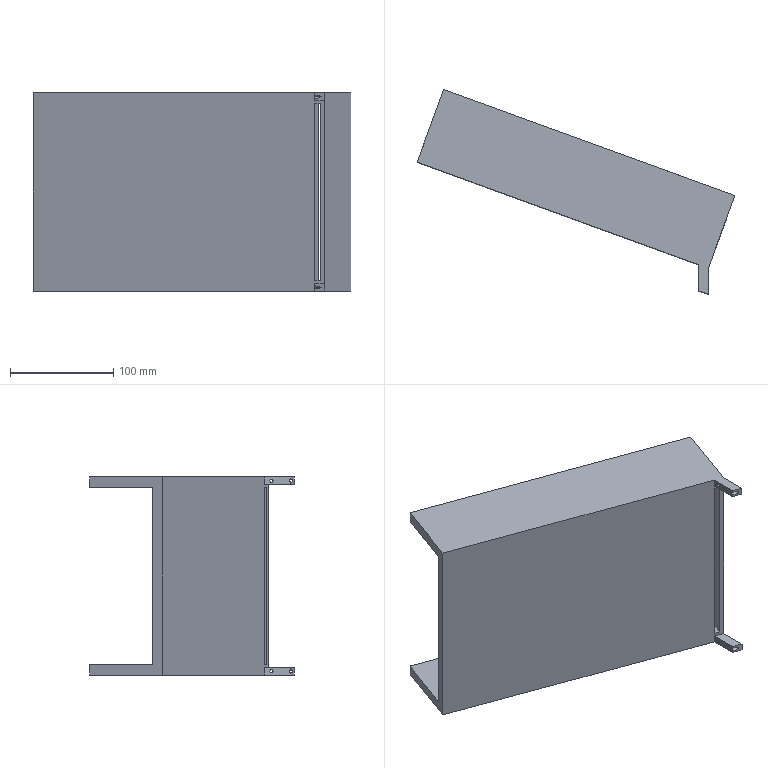Part | SolidWorks | features SplitBody 1 | 1 solid | 27 faces | box 307.559 x 198.283 x 191.8 mm | volume 1005871 mm3 | plane 19 | cylinder 8 | commonest cylinder face diameters 3 x8
STEP:
#1=CARTESIAN_POINT('',(-94.922,250.959,-452.616));
#2=VERTEX_POINT('',#1);
#3=CARTESIAN_POINT('',(-94.922,253.959,-452.616));
#4=VERTEX_POINT('',#3);
#5=CARTESIAN_POINT('',(-94.922,252.459,-452.616));
#6=DIRECTION('',(-1.,0.,0.));
#7=DIRECTION('',(0.,1.,0.));
#8=AXIS2_PLACEMENT_3D('',#5,#6,#7);
#9=CIRCLE('',#8,1.5);
#10=EDGE_CURVE('',#2,#4,#9,.T.);
#11=ORIENTED_EDGE('',*,*,#10,.T.);
#12=CARTESIAN_POINT('',(-85.525,253.959,-452.616));
#13=VERTEX_POINT('',#12);
#14=CARTESIAN_POINT('',(-88.525,253.959,-452.616));
#15=DIRECTION('',(1.,0.,0.));
#16=VECTOR('',#15,1000.);
#17=LINE('',#14,#16);
#18=EDGE_CURVE('',#4,#13,#17,.T.);
#19=ORIENTED_EDGE('',*,*,#18,.T.);
#20=CARTESIAN_POINT('',(-85.525,250.959,-452.616));
#21=VERTEX_POINT('',#20);
#22=CARTESIAN_POINT('',(-85.525,252.459,-452.616));
#23=DIRECTION('',(1.,0.,0.));
#24=DIRECTION('',(0.,-1.,0.));
#25=AXIS2_PLACEMENT_3D('',#22,#23,#24);
#26=CIRCLE('',#25,1.5);
#27=EDGE_CURVE('',#13,#21,#26,.T.);
#28=ORIENTED_EDGE('',*,*,#27,.T.);
#29=CARTESIAN_POINT('',(-88.525,250.959,-452.616));
#30=DIRECTION('',(1.,0.,0.));
#31=VECTOR('',#30,1000.);
#32=LINE('',#29,#31);
#33=EDGE_CURVE('',#2,#21,#32,.T.);
#34=ORIENTED_EDGE('',*,*,#33,.F.);
#35=EDGE_LOOP('',(#11,#19,#28,#34));
#36=FACE_OUTER_BOUND('',#35,.T.);
#37=CARTESIAN_POINT('',(-88.525,252.459,-452.616));
#38=DIRECTION('',(1.,0.,0.));
#39=DIRECTION('',(0.,-1.,0.));
#40=AXIS2_PLACEMENT_3D('',#37,#38,#39);
#41=CYLINDRICAL_SURFACE('',#40,1.5);
#42=ADVANCED_FACE('',(#36),#41,.F.);
#43=CARTESIAN_POINT('',(-94.922,233.679,-451.176));
#44=VERTEX_POINT('',#43);
#45=CARTESIAN_POINT('',(-94.922,234.759,-452.616));
#46=VERTEX_POINT('',#45);
#47=CARTESIAN_POINT('',(-94.922,233.259,-452.616));
#48=DIRECTION('',(-1.,0.,0.));
#49=DIRECTION('',(0.,1.,0.));
#50=AXIS2_PLACEMENT_3D('',#47,#48,#49);
#51=CIRCLE('',#50,1.5);
#52=EDGE_CURVE('',#44,#46,#51,.T.);
#53=ORIENTED_EDGE('',*,*,#52,.T.);
#54=CARTESIAN_POINT('',(-85.525,234.759,-452.616));
#55=VERTEX_POINT('',#54);
#56=CARTESIAN_POINT('',(-88.525,234.759,-452.616));
#57=DIRECTION('',(1.,0.,0.));
#58=VECTOR('',#57,1000.);
#59=LINE('',#56,#58);
#60=EDGE_CURVE('',#46,#55,#59,.T.);
#61=ORIENTED_EDGE('',*,*,#60,.T.);
#62=CARTESIAN_POINT('',(-85.525,231.759,-452.616));
#63=VERTEX_POINT('',#62);
#64=CARTESIAN_POINT('',(-85.525,233.259,-452.616));
#65=DIRECTION('',(1.,0.,0.));
#66=DIRECTION('',(0.,-1.,0.));
#67=AXIS2_PLACEMENT_3D('',#64,#65,#66);
#68=CIRCLE('',#67,1.5);
#69=EDGE_CURVE('',#55,#63,#68,.T.);
#70=ORIENTED_EDGE('',*,*,#69,.T.);
#71=CARTESIAN_POINT('',(-89.646,231.759,-452.616));
#72=VERTEX_POINT('',#71);
#73=CARTESIAN_POINT('',(-88.525,231.759,-452.616));
#74=DIRECTION('',(1.,0.,0.));
#75=VECTOR('',#74,1000.);
#76=LINE('',#73,#75);
#77=EDGE_CURVE('',#72,#63,#76,.T.);
#78=ORIENTED_EDGE('',*,*,#77,.F.);
#79=CARTESIAN_POINT('',(-89.646,231.759,-452.616));
#80=CARTESIAN_POINT('',(-89.646,231.759,-451.525));
#81=CARTESIAN_POINT('',(-92.044,232.632,-450.87));
#82=CARTESIAN_POINT('',(-94.922,233.679,-451.176));
#83=(BOUNDED_CURVE()B_SPLINE_CURVE(3,(#79,#80,#81,#82),.UNSPECIFIED.,.F.,.F.)B_SPLINE_CURVE_WITH_KNOTS((4,4),(0.,1.855),.UNSPECIFIED.)CURVE()GEOMETRIC_REPRESENTATION_ITEM()RATIONAL_B_SPLINE_CURVE((1.,0.7333,0.7333,1.))REPRESENTATION_ITEM(''));
#84=EDGE_CURVE('',#72,#44,#83,.T.);
#85=ORIENTED_EDGE('',*,*,#84,.T.);
#86=EDGE_LOOP('',(#53,#61,#70,#78,#85));
#87=FACE_OUTER_BOUND('',#86,.T.);
#88=CARTESIAN_POINT('',(-88.525,233.259,-452.616));
#89=DIRECTION('',(1.,0.,0.));
#90=DIRECTION('',(0.,-1.,0.));
#91=AXIS2_PLACEMENT_3D('',#88,#89,#90);
#92=CYLINDRICAL_SURFACE('',#91,1.5);
#93=ADVANCED_FACE('',(#87),#92,.F.);
#94=CARTESIAN_POINT('',(-94.922,250.959,-267.816));
#95=VERTEX_POINT('',#94);
#96=CARTESIAN_POINT('',(-94.922,253.959,-267.816));
#97=VERTEX_POINT('',#96);
#98=CARTESIAN_POINT('',(-94.922,252.459,-267.816));
#99=DIRECTION('',(-1.,0.,0.));
#100=DIRECTION('',(0.,1.,0.));
#101=AXIS2_PLACEMENT_3D('',#98,#99,#100);
#102=CIRCLE('',#101,1.5);
#103=EDGE_CURVE('',#95,#97,#102,.T.);
#104=ORIENTED_EDGE('',*,*,#103,.T.);
#105=CARTESIAN_POINT('',(-85.525,253.959,-267.816));
#106=VERTEX_POINT('',#105);
#107=CARTESIAN_POINT('',(-88.525,253.959,-267.816));
#108=DIRECTION('',(1.,0.,0.));
#109=VECTOR('',#108,1000.);
#110=LINE('',#107,#109);
#111=EDGE_CURVE('',#97,#106,#110,.T.);
#112=ORIENTED_EDGE('',*,*,#111,.T.);
#113=CARTESIAN_POINT('',(-85.525,250.959,-267.816));
#114=VERTEX_POINT('',#113);
#115=CARTESIAN_POINT('',(-85.525,252.459,-267.816));
#116=DIRECTION('',(1.,0.,0.));
#117=DIRECTION('',(0.,-1.,0.));
#118=AXIS2_PLACEMENT_3D('',#115,#116,#117);
#119=CIRCLE('',#118,1.5);
#120=EDGE_CURVE('',#106,#114,#119,.T.);
#121=ORIENTED_EDGE('',*,*,#120,.T.);
#122=CARTESIAN_POINT('',(-88.525,250.959,-267.816));
#123=DIRECTION('',(1.,0.,0.));
#124=VECTOR('',#123,1000.);
#125=LINE('',#122,#124);
#126=EDGE_CURVE('',#95,#114,#125,.T.);
#127=ORIENTED_EDGE('',*,*,#126,.F.);
#128=EDGE_LOOP('',(#104,#112,#121,#127));
#129=FACE_OUTER_BOUND('',#128,.T.);
#130=CARTESIAN_POINT('',(-88.525,252.459,-267.816));
#131=DIRECTION('',(1.,0.,0.));
#132=DIRECTION('',(0.,-1.,0.));
#133=AXIS2_PLACEMENT_3D('',#130,#131,#132);
#134=CYLINDRICAL_SURFACE('',#133,1.5);
#135=ADVANCED_FACE('',(#129),#134,.F.);
#136=CARTESIAN_POINT('',(-94.922,233.679,-266.376));
#137=VERTEX_POINT('',#136);
#138=CARTESIAN_POINT('',(-94.922,234.759,-267.816));
#139=VERTEX_POINT('',#138);
#140=CARTESIAN_POINT('',(-94.922,233.259,-267.816));
#141=DIRECTION('',(-1.,0.,0.));
#142=DIRECTION('',(0.,1.,0.));
#143=AXIS2_PLACEMENT_3D('',#140,#141,#142);
#144=CIRCLE('',#143,1.5);
#145=EDGE_CURVE('',#137,#139,#144,.T.);
#146=ORIENTED_EDGE('',*,*,#145,.T.);
#147=CARTESIAN_POINT('',(-85.525,234.759,-267.816));
#148=VERTEX_POINT('',#147);
#149=CARTESIAN_POINT('',(-88.525,234.759,-267.816));
#150=DIRECTION('',(1.,0.,0.));
#151=VECTOR('',#150,1000.);
#152=LINE('',#149,#151);
#153=EDGE_CURVE('',#139,#148,#152,.T.);
#154=ORIENTED_EDGE('',*,*,#153,.T.);
#155=CARTESIAN_POINT('',(-85.525,231.759,-267.816));
#156=VERTEX_POINT('',#155);
#157=CARTESIAN_POINT('',(-85.525,233.259,-267.816));
#158=DIRECTION('',(1.,0.,0.));
#159=DIRECTION('',(0.,-1.,0.));
#160=AXIS2_PLACEMENT_3D('',#157,#158,#159);
#161=CIRCLE('',#160,1.5);
#162=EDGE_CURVE('',#148,#156,#161,.T.);
#163=ORIENTED_EDGE('',*,*,#162,.T.);
#164=CARTESIAN_POINT('',(-89.646,231.759,-267.816));
#165=VERTEX_POINT('',#164);
#166=CARTESIAN_POINT('',(-88.525,231.759,-267.816));
#167=DIRECTION('',(1.,0.,0.));
#168=VECTOR('',#167,1000.);
#169=LINE('',#166,#168);
#170=EDGE_CURVE('',#165,#156,#169,.T.);
#171=ORIENTED_EDGE('',*,*,#170,.F.);
#172=CARTESIAN_POINT('',(-89.646,231.759,-267.816));
#173=CARTESIAN_POINT('',(-89.646,231.759,-266.725));
#174=CARTESIAN_POINT('',(-92.044,232.632,-266.07));
#175=CARTESIAN_POINT('',(-94.922,233.679,-266.376));
#176=(BOUNDED_CURVE()B_SPLINE_CURVE(3,(#172,#173,#174,#175),.UNSPECIFIED.,.F.,.F.)B_SPLINE_CURVE_WITH_KNOTS((4,4),(0.,1.855),.UNSPECIFIED.)CURVE()GEOMETRIC_REPRESENTATION_ITEM()RATIONAL_B_SPLINE_CURVE((1.,0.7333,0.7333,1.))REPRESENTATION_ITEM(''));
#177=EDGE_CURVE('',#165,#137,#176,.T.);
#178=ORIENTED_EDGE('',*,*,#177,.T.);
#179=EDGE_LOOP('',(#146,#154,#163,#171,#178));
#180=FACE_OUTER_BOUND('',#179,.T.);
#181=CARTESIAN_POINT('',(-88.525,233.259,-267.816));
#182=DIRECTION('',(1.,0.,0.));
#183=DIRECTION('',(0.,-1.,0.));
#184=AXIS2_PLACEMENT_3D('',#181,#182,#183);
#185=CYLINDRICAL_SURFACE('',#184,1.5);
#186=ADVANCED_FACE('',(#180),#185,.F.);
#187=CARTESIAN_POINT('',(-341.781,428.542,-274.316));
#188=VERTEX_POINT('',#187);
#189=CARTESIAN_POINT('',(-341.781,428.542,-264.316));
#190=VERTEX_POINT('',#189);
#191=CARTESIAN_POINT('',(-341.781,428.542,-456.116));
#192=DIRECTION('',(0.,0.,1.));
#193=VECTOR('',#192,1000.);
#194=LINE('',#191,#193);
#195=EDGE_CURVE('',#188,#190,#194,.T.);
#196=ORIENTED_EDGE('',*,*,#195,.F.);
#197=CARTESIAN_POINT('',(-364.012,367.462,-274.316));
#198=VERTEX_POINT('',#197);
#199=CARTESIAN_POINT('',(-341.781,428.542,-274.316));
#200=DIRECTION('',(-0.342,-0.9397,0.));
#201=VECTOR('',#200,1000.);
#202=LINE('',#199,#201);
#203=EDGE_CURVE('',#188,#198,#202,.T.);
#204=ORIENTED_EDGE('',*,*,#203,.T.);
#205=CARTESIAN_POINT('',(-364.012,367.462,-446.116));
#206=VERTEX_POINT('',#205);
#207=CARTESIAN_POINT('',(-364.012,367.462,-456.116));
#208=DIRECTION('',(0.,0.,1.));
#209=VECTOR('',#208,1000.);
#210=LINE('',#207,#209);
#211=EDGE_CURVE('',#206,#198,#210,.T.);
#212=ORIENTED_EDGE('',*,*,#211,.F.);
#213=CARTESIAN_POINT('',(-341.781,428.542,-446.116));
#214=VERTEX_POINT('',#213);
#215=CARTESIAN_POINT('',(-341.781,428.542,-446.116));
#216=DIRECTION('',(-0.342,-0.9397,0.));
#217=VECTOR('',#216,1000.);
#218=LINE('',#215,#217);
#219=EDGE_CURVE('',#214,#206,#218,.T.);
#220=ORIENTED_EDGE('',*,*,#219,.F.);
#221=CARTESIAN_POINT('',(-341.781,428.542,-456.116));
#222=VERTEX_POINT('',#221);
#223=CARTESIAN_POINT('',(-341.781,428.542,-456.116));
#224=DIRECTION('',(0.,0.,1.));
#225=VECTOR('',#224,1000.);
#226=LINE('',#223,#225);
#227=EDGE_CURVE('',#222,#214,#226,.T.);
#228=ORIENTED_EDGE('',*,*,#227,.F.);
#229=CARTESIAN_POINT('',(-367.432,358.065,-456.116));
#230=VERTEX_POINT('',#229);
#231=CARTESIAN_POINT('',(-341.781,428.542,-456.116));
#232=DIRECTION('',(-0.342,-0.9397,0.));
#233=VECTOR('',#232,1000.);
#234=LINE('',#231,#233);
#235=EDGE_CURVE('',#222,#230,#234,.T.);
#236=ORIENTED_EDGE('',*,*,#235,.T.);
#237=CARTESIAN_POINT('',(-367.432,358.065,-264.316));
#238=VERTEX_POINT('',#237);
#239=CARTESIAN_POINT('',(-367.432,358.065,-456.116));
#240=DIRECTION('',(0.,0.,1.));
#241=VECTOR('',#240,1000.);
#242=LINE('',#239,#241);
#243=EDGE_CURVE('',#230,#238,#242,.T.);
#244=ORIENTED_EDGE('',*,*,#243,.T.);
#245=CARTESIAN_POINT('',(-341.781,428.542,-264.316));
#246=DIRECTION('',(-0.342,-0.9397,0.));
#247=VECTOR('',#246,1000.);
#248=LINE('',#245,#247);
#249=EDGE_CURVE('',#190,#238,#248,.T.);
#250=ORIENTED_EDGE('',*,*,#249,.F.);
#251=EDGE_LOOP('',(#196,#204,#212,#220,#228,#236,#244,#250));
#252=FACE_OUTER_BOUND('',#251,.T.);
#253=CARTESIAN_POINT('',(-341.781,428.542,-456.116));
#254=DIRECTION('',(0.9397,-0.342,0.));
#255=DIRECTION('',(-0.342,-0.9397,0.));
#256=AXIS2_PLACEMENT_3D('',#253,#254,#255);
#257=PLANE('',#256);
#258=ADVANCED_FACE('',(#252),#257,.F.);
#259=CARTESIAN_POINT('',(-94.922,258.879,-264.316));
#260=VERTEX_POINT('',#259);
#261=CARTESIAN_POINT('',(-367.432,358.065,-264.316));
#262=DIRECTION('',(0.9397,-0.342,0.));
#263=VECTOR('',#262,1000.);
#264=LINE('',#261,#263);
#265=EDGE_CURVE('',#238,#260,#264,.T.);
#266=ORIENTED_EDGE('',*,*,#265,.T.);
#267=CARTESIAN_POINT('',(-94.922,233.679,-264.316));
#268=VERTEX_POINT('',#267);
#269=CARTESIAN_POINT('',(-94.922,258.879,-264.316));
#270=DIRECTION('',(0.,-1.,0.));
#271=VECTOR('',#270,1000.);
#272=LINE('',#269,#271);
#273=EDGE_CURVE('',#260,#268,#272,.T.);
#274=ORIENTED_EDGE('',*,*,#273,.T.);
#275=CARTESIAN_POINT('',(-85.525,230.259,-264.316));
#276=VERTEX_POINT('',#275);
#277=CARTESIAN_POINT('',(-85.525,230.259,-264.316));
#278=DIRECTION('',(0.9397,-0.342,0.));
#279=VECTOR('',#278,1000.);
#280=LINE('',#277,#279);
#281=EDGE_CURVE('',#268,#276,#280,.T.);
#282=ORIENTED_EDGE('',*,*,#281,.T.);
#283=CARTESIAN_POINT('',(-85.525,255.459,-264.316));
#284=VERTEX_POINT('',#283);
#285=CARTESIAN_POINT('',(-85.525,255.459,-264.316));
#286=DIRECTION('',(0.,1.,0.));
#287=VECTOR('',#286,1000.);
#288=LINE('',#285,#287);
#289=EDGE_CURVE('',#276,#284,#288,.T.);
#290=ORIENTED_EDGE('',*,*,#289,.T.);
#291=CARTESIAN_POINT('',(-59.873,325.936,-264.316));
#292=VERTEX_POINT('',#291);
#293=CARTESIAN_POINT('',(-59.873,325.936,-264.316));
#294=DIRECTION('',(-0.342,-0.9397,0.));
#295=VECTOR('',#294,1000.);
#296=LINE('',#293,#295);
#297=EDGE_CURVE('',#292,#284,#296,.T.);
#298=ORIENTED_EDGE('',*,*,#297,.F.);
#299=CARTESIAN_POINT('',(-341.781,428.542,-264.316));
#300=DIRECTION('',(0.9397,-0.342,0.));
#301=VECTOR('',#300,1000.);
#302=LINE('',#299,#301);
#303=EDGE_CURVE('',#190,#292,#302,.T.);
#304=ORIENTED_EDGE('',*,*,#303,.F.);
#305=ORIENTED_EDGE('',*,*,#249,.T.);
#306=EDGE_LOOP('',(#266,#274,#282,#290,#298,#304,#305));
#307=FACE_OUTER_BOUND('',#306,.T.);
#308=CARTESIAN_POINT('',(-341.781,428.542,-264.316));
#309=DIRECTION('',(0.,0.,-1.));
#310=DIRECTION('',(-0.9397,0.342,0.));
#311=AXIS2_PLACEMENT_3D('',#308,#309,#310);
#312=PLANE('',#311);
#313=ADVANCED_FACE('',(#307),#312,.F.);
#314=CARTESIAN_POINT('',(-85.525,255.459,-271.316));
#315=VERTEX_POINT('',#314);
#316=CARTESIAN_POINT('',(-85.525,255.459,-456.116));
#317=DIRECTION('',(0.,0.,-1.));
#318=VECTOR('',#317,1000.);
#319=LINE('',#316,#318);
#320=EDGE_CURVE('',#284,#315,#319,.T.);
#321=ORIENTED_EDGE('',*,*,#320,.T.);
#322=CARTESIAN_POINT('',(-85.525,255.459,-449.116));
#323=VERTEX_POINT('',#322);
#324=CARTESIAN_POINT('',(-85.525,255.459,-456.116));
#325=DIRECTION('',(0.,0.,-1.));
#326=VECTOR('',#325,1000.);
#327=LINE('',#324,#326);
#328=EDGE_CURVE('',#315,#323,#327,.T.);
#329=ORIENTED_EDGE('',*,*,#328,.T.);
#330=CARTESIAN_POINT('',(-85.525,255.459,-456.116));
#331=VERTEX_POINT('',#330);
#332=CARTESIAN_POINT('',(-85.525,255.459,-449.116));
#333=DIRECTION('',(0.,0.,-1.));
#334=VECTOR('',#333,1000.);
#335=LINE('',#332,#334);
#336=EDGE_CURVE('',#323,#331,#335,.T.);
#337=ORIENTED_EDGE('',*,*,#336,.T.);
#338=CARTESIAN_POINT('',(-59.873,325.936,-456.116));
#339=VERTEX_POINT('',#338);
#340=CARTESIAN_POINT('',(-59.873,325.936,-456.116));
#341=DIRECTION('',(-0.342,-0.9397,0.));
#342=VECTOR('',#341,1000.);
#343=LINE('',#340,#342);
#344=EDGE_CURVE('',#339,#331,#343,.T.);
#345=ORIENTED_EDGE('',*,*,#344,.F.);
#346=CARTESIAN_POINT('',(-59.873,325.936,-456.116));
#347=DIRECTION('',(0.,0.,-1.));
#348=VECTOR('',#347,1000.);
#349=LINE('',#346,#348);
#350=EDGE_CURVE('',#292,#339,#349,.T.);
#351=ORIENTED_EDGE('',*,*,#350,.F.);
#352=ORIENTED_EDGE('',*,*,#297,.T.);
#353=EDGE_LOOP('',(#321,#329,#337,#345,#351,#352));
#354=FACE_OUTER_BOUND('',#353,.T.);
#355=CARTESIAN_POINT('',(-59.873,325.936,-456.116));
#356=DIRECTION('',(-0.9397,0.342,0.));
#357=DIRECTION('',(0.342,0.9397,0.));
#358=AXIS2_PLACEMENT_3D('',#355,#356,#357);
#359=PLANE('',#358);
#360=ADVANCED_FACE('',(#354),#359,.F.);
#361=ORIENTED_EDGE('',*,*,#344,.T.);
#362=CARTESIAN_POINT('',(-85.525,230.259,-456.116));
#363=VERTEX_POINT('',#362);
#364=CARTESIAN_POINT('',(-85.525,230.259,-456.116));
#365=DIRECTION('',(0.,-1.,0.));
#366=VECTOR('',#365,1000.);
#367=LINE('',#364,#366);
#368=EDGE_CURVE('',#331,#363,#367,.T.);
#369=ORIENTED_EDGE('',*,*,#368,.T.);
#370=CARTESIAN_POINT('',(-94.922,233.679,-456.116));
#371=VERTEX_POINT('',#370);
#372=CARTESIAN_POINT('',(-94.922,233.679,-456.116));
#373=DIRECTION('',(-0.9397,0.342,0.));
#374=VECTOR('',#373,1000.);
#375=LINE('',#372,#374);
#376=EDGE_CURVE('',#363,#371,#375,.T.);
#377=ORIENTED_EDGE('',*,*,#376,.T.);
#378=CARTESIAN_POINT('',(-94.922,258.879,-456.116));
#379=VERTEX_POINT('',#378);
#380=CARTESIAN_POINT('',(-94.922,258.879,-456.116));
#381=DIRECTION('',(0.,1.,0.));
#382=VECTOR('',#381,1000.);
#383=LINE('',#380,#382);
#384=EDGE_CURVE('',#371,#379,#383,.T.);
#385=ORIENTED_EDGE('',*,*,#384,.T.);
#386=CARTESIAN_POINT('',(-367.432,358.065,-456.116));
#387=DIRECTION('',(-0.9397,0.342,0.));
#388=VECTOR('',#387,1000.);
#389=LINE('',#386,#388);
#390=EDGE_CURVE('',#379,#230,#389,.T.);
#391=ORIENTED_EDGE('',*,*,#390,.T.);
#392=ORIENTED_EDGE('',*,*,#235,.F.);
#393=CARTESIAN_POINT('',(-341.781,428.542,-456.116));
#394=DIRECTION('',(-0.9397,0.342,0.));
#395=VECTOR('',#394,1000.);
#396=LINE('',#393,#395);
#397=EDGE_CURVE('',#339,#222,#396,.T.);
#398=ORIENTED_EDGE('',*,*,#397,.F.);
#399=EDGE_LOOP('',(#361,#369,#377,#385,#391,#392,#398));
#400=FACE_OUTER_BOUND('',#399,.T.);
#401=CARTESIAN_POINT('',(-341.781,428.542,-456.116));
#402=DIRECTION('',(0.,0.,1.));
#403=DIRECTION('',(-0.342,-0.9397,0.));
#404=AXIS2_PLACEMENT_3D('',#401,#402,#403);
#405=PLANE('',#404);
#406=ADVANCED_FACE('',(#400),#405,.F.);
#407=CARTESIAN_POINT('',(-63.854,327.385,-446.116));
#408=VERTEX_POINT('',#407);
#409=CARTESIAN_POINT('',(-341.781,428.542,-446.116));
#410=DIRECTION('',(-0.9397,0.342,0.));
#411=VECTOR('',#410,1000.);
#412=LINE('',#409,#411);
#413=EDGE_CURVE('',#408,#214,#412,.T.);
#414=ORIENTED_EDGE('',*,*,#413,.F.);
#415=CARTESIAN_POINT('',(-63.854,327.385,-274.316));
#416=VERTEX_POINT('',#415);
#417=CARTESIAN_POINT('',(-63.854,327.385,-446.116));
#418=DIRECTION('',(0.,0.,-1.));
#419=VECTOR('',#418,1000.);
#420=LINE('',#417,#419);
#421=EDGE_CURVE('',#416,#408,#420,.T.);
#422=ORIENTED_EDGE('',*,*,#421,.F.);
#423=CARTESIAN_POINT('',(-341.781,428.542,-274.316));
#424=DIRECTION('',(0.9397,-0.342,0.));
#425=VECTOR('',#424,1000.);
#426=LINE('',#423,#425);
#427=EDGE_CURVE('',#188,#416,#426,.T.);
#428=ORIENTED_EDGE('',*,*,#427,.F.);
#429=ORIENTED_EDGE('',*,*,#195,.T.);
#430=ORIENTED_EDGE('',*,*,#303,.T.);
#431=ORIENTED_EDGE('',*,*,#350,.T.);
#432=ORIENTED_EDGE('',*,*,#397,.T.);
#433=ORIENTED_EDGE('',*,*,#227,.T.);
#434=EDGE_LOOP('',(#414,#422,#428,#429,#430,#431,#432,#433));
#435=FACE_OUTER_BOUND('',#434,.T.);
#436=CARTESIAN_POINT('',(-213.116,381.712,-370.539));
#437=DIRECTION('',(0.342,0.9397,0.));
#438=DIRECTION('',(0.9397,-0.342,0.));
#439=AXIS2_PLACEMENT_3D('',#436,#437,#438);
#440=PLANE('',#439);
#441=ADVANCED_FACE('',(#435),#440,.T.);
#442=CARTESIAN_POINT('',(-89.505,256.908,-446.116));
#443=VERTEX_POINT('',#442);
#444=CARTESIAN_POINT('',(-94.922,258.879,-446.116));
#445=VERTEX_POINT('',#444);
#446=CARTESIAN_POINT('',(-238.768,311.235,-446.116));
#447=DIRECTION('',(-0.9397,0.342,0.));
#448=VECTOR('',#447,1000.);
#449=LINE('',#446,#448);
#450=EDGE_CURVE('',#443,#445,#449,.T.);
#451=ORIENTED_EDGE('',*,*,#450,.T.);
#452=CARTESIAN_POINT('',(-94.922,258.879,-274.316));
#453=VERTEX_POINT('',#452);
#454=CARTESIAN_POINT('',(-94.922,258.879,-370.539));
#455=DIRECTION('',(0.,0.,1.));
#456=VECTOR('',#455,1000.);
#457=LINE('',#454,#456);
#458=EDGE_CURVE('',#445,#453,#457,.T.);
#459=ORIENTED_EDGE('',*,*,#458,.T.);
#460=CARTESIAN_POINT('',(-89.505,256.908,-274.316));
#461=VERTEX_POINT('',#460);
#462=CARTESIAN_POINT('',(-238.768,311.235,-274.316));
#463=DIRECTION('',(0.9397,-0.342,0.));
#464=VECTOR('',#463,1000.);
#465=LINE('',#462,#464);
#466=EDGE_CURVE('',#453,#461,#465,.T.);
#467=ORIENTED_EDGE('',*,*,#466,.T.);
#468=CARTESIAN_POINT('',(-89.505,256.908,-370.539));
#469=DIRECTION('',(0.,0.,-1.));
#470=VECTOR('',#469,1000.);
#471=LINE('',#468,#470);
#472=EDGE_CURVE('',#461,#443,#471,.T.);
#473=ORIENTED_EDGE('',*,*,#472,.T.);
#474=EDGE_LOOP('',(#451,#459,#467,#473));
#475=FACE_BOUND('',#474,.T.);
#476=ORIENTED_EDGE('',*,*,#390,.F.);
#477=CARTESIAN_POINT('',(-94.922,258.879,-449.116));
#478=VERTEX_POINT('',#477);
#479=CARTESIAN_POINT('',(-94.922,258.879,-449.116));
#480=DIRECTION('',(0.,0.,-1.));
#481=VECTOR('',#480,1000.);
#482=LINE('',#479,#481);
#483=EDGE_CURVE('',#478,#379,#482,.T.);
#484=ORIENTED_EDGE('',*,*,#483,.F.);
#485=CARTESIAN_POINT('',(-85.525,255.459,-449.116));
#486=DIRECTION('',(0.9397,-0.342,0.));
#487=VECTOR('',#486,1000.);
#488=LINE('',#485,#487);
#489=EDGE_CURVE('',#478,#323,#488,.T.);
#490=ORIENTED_EDGE('',*,*,#489,.T.);
#491=ORIENTED_EDGE('',*,*,#328,.F.);
#492=CARTESIAN_POINT('',(-94.922,258.879,-271.316));
#493=VERTEX_POINT('',#492);
#494=CARTESIAN_POINT('',(-85.525,255.459,-271.316));
#495=DIRECTION('',(-0.9397,0.342,0.));
#496=VECTOR('',#495,1000.);
#497=LINE('',#494,#496);
#498=EDGE_CURVE('',#315,#493,#497,.T.);
#499=ORIENTED_EDGE('',*,*,#498,.T.);
#500=CARTESIAN_POINT('',(-94.922,258.879,-271.316));
#501=DIRECTION('',(0.,0.,1.));
#502=VECTOR('',#501,1000.);
#503=LINE('',#500,#502);
#504=EDGE_CURVE('',#493,#260,#503,.T.);
#505=ORIENTED_EDGE('',*,*,#504,.T.);
#506=ORIENTED_EDGE('',*,*,#265,.F.);
#507=ORIENTED_EDGE('',*,*,#243,.F.);
#508=EDGE_LOOP('',(#476,#484,#490,#491,#499,#505,#506,#507));
#509=FACE_OUTER_BOUND('',#508,.T.);
#510=CARTESIAN_POINT('',(-238.768,311.235,-370.539));
#511=DIRECTION('',(0.342,0.9397,0.));
#512=DIRECTION('',(0.9397,-0.342,0.));
#513=AXIS2_PLACEMENT_3D('',#510,#511,#512);
#514=PLANE('',#513);
#515=ADVANCED_FACE('',(#475,#509),#514,.F.);
#516=CARTESIAN_POINT('',(-91.501,268.276,-274.316));
#517=VERTEX_POINT('',#516);
#518=CARTESIAN_POINT('',(-364.012,367.462,-274.316));
#519=DIRECTION('',(0.9397,-0.342,0.));
#520=VECTOR('',#519,1000.);
#521=LINE('',#518,#520);
#522=EDGE_CURVE('',#198,#517,#521,.T.);
#523=ORIENTED_EDGE('',*,*,#522,.F.);
#524=ORIENTED_EDGE('',*,*,#203,.F.);
#525=ORIENTED_EDGE('',*,*,#427,.T.);
#526=CARTESIAN_POINT('',(-94.635,242.812,-274.316));
#527=DIRECTION('',(0.342,0.9397,0.));
#528=VECTOR('',#527,1000.);
#529=LINE('',#526,#528);
#530=EDGE_CURVE('',#461,#416,#529,.T.);
#531=ORIENTED_EDGE('',*,*,#530,.F.);
#532=ORIENTED_EDGE('',*,*,#466,.F.);
#533=CARTESIAN_POINT('',(-100.052,244.784,-274.316));
#534=DIRECTION('',(0.342,0.9397,0.));
#535=VECTOR('',#534,1000.);
#536=LINE('',#533,#535);
#537=EDGE_CURVE('',#453,#517,#536,.T.);
#538=ORIENTED_EDGE('',*,*,#537,.T.);
#539=EDGE_LOOP('',(#523,#524,#525,#531,#532,#538));
#540=FACE_OUTER_BOUND('',#539,.T.);
#541=CARTESIAN_POINT('',(-341.781,428.542,-274.316));
#542=DIRECTION('',(0.,0.,-1.));
#543=DIRECTION('',(-0.9397,0.342,0.));
#544=AXIS2_PLACEMENT_3D('',#541,#542,#543);
#545=PLANE('',#544);
#546=ADVANCED_FACE('',(#540),#545,.T.);
#547=CARTESIAN_POINT('',(-91.501,268.276,-446.116));
#548=VERTEX_POINT('',#547);
#549=CARTESIAN_POINT('',(-364.012,367.462,-446.116));
#550=DIRECTION('',(-0.9397,0.342,0.));
#551=VECTOR('',#550,1000.);
#552=LINE('',#549,#551);
#553=EDGE_CURVE('',#548,#206,#552,.T.);
#554=ORIENTED_EDGE('',*,*,#553,.F.);
#555=CARTESIAN_POINT('',(-100.052,244.784,-446.116));
#556=DIRECTION('',(0.342,0.9397,0.));
#557=VECTOR('',#556,1000.);
#558=LINE('',#555,#557);
#559=EDGE_CURVE('',#445,#548,#558,.T.);
#560=ORIENTED_EDGE('',*,*,#559,.F.);
#561=ORIENTED_EDGE('',*,*,#450,.F.);
#562=CARTESIAN_POINT('',(-94.635,242.812,-446.116));
#563=DIRECTION('',(0.342,0.9397,0.));
#564=VECTOR('',#563,1000.);
#565=LINE('',#562,#564);
#566=EDGE_CURVE('',#443,#408,#565,.T.);
#567=ORIENTED_EDGE('',*,*,#566,.T.);
#568=ORIENTED_EDGE('',*,*,#413,.T.);
#569=ORIENTED_EDGE('',*,*,#219,.T.);
#570=EDGE_LOOP('',(#554,#560,#561,#567,#568,#569));
#571=FACE_OUTER_BOUND('',#570,.T.);
#572=CARTESIAN_POINT('',(-341.781,428.542,-446.116));
#573=DIRECTION('',(0.,0.,1.));
#574=DIRECTION('',(-0.342,-0.9397,0.));
#575=AXIS2_PLACEMENT_3D('',#572,#573,#574);
#576=PLANE('',#575);
#577=ADVANCED_FACE('',(#571),#576,.T.);
#578=ORIENTED_EDGE('',*,*,#211,.T.);
#579=ORIENTED_EDGE('',*,*,#522,.T.);
#580=CARTESIAN_POINT('',(-91.501,268.276,-456.116));
#581=DIRECTION('',(0.,0.,-1.));
#582=VECTOR('',#581,1000.);
#583=LINE('',#580,#582);
#584=EDGE_CURVE('',#517,#548,#583,.T.);
#585=ORIENTED_EDGE('',*,*,#584,.T.);
#586=ORIENTED_EDGE('',*,*,#553,.T.);
#587=EDGE_LOOP('',(#578,#579,#585,#586));
#588=FACE_OUTER_BOUND('',#587,.T.);
#589=CARTESIAN_POINT('',(-235.347,320.632,-370.539));
#590=DIRECTION('',(0.342,0.9397,0.));
#591=DIRECTION('',(0.9397,-0.342,0.));
#592=AXIS2_PLACEMENT_3D('',#589,#590,#591);
#593=PLANE('',#592);
#594=ADVANCED_FACE('',(#588),#593,.T.);
#595=CARTESIAN_POINT('',(-85.525,252.459,-267.816));
#596=DIRECTION('',(1.,0.,0.));
#597=DIRECTION('',(0.,-1.,0.));
#598=AXIS2_PLACEMENT_3D('',#595,#596,#597);
#599=CIRCLE('',#598,1.5);
#600=EDGE_CURVE('',#114,#106,#599,.T.);
#601=ORIENTED_EDGE('',*,*,#600,.F.);
#602=ORIENTED_EDGE('',*,*,#120,.F.);
#603=EDGE_LOOP('',(#601,#602));
#604=FACE_BOUND('',#603,.T.);
#605=CARTESIAN_POINT('',(-85.525,233.259,-267.816));
#606=DIRECTION('',(1.,0.,0.));
#607=DIRECTION('',(0.,-1.,0.));
#608=AXIS2_PLACEMENT_3D('',#605,#606,#607);
#609=CIRCLE('',#608,1.5);
#610=EDGE_CURVE('',#156,#148,#609,.T.);
#611=ORIENTED_EDGE('',*,*,#610,.F.);
#612=ORIENTED_EDGE('',*,*,#162,.F.);
#613=EDGE_LOOP('',(#611,#612));
#614=FACE_BOUND('',#613,.T.);
#615=ORIENTED_EDGE('',*,*,#289,.F.);
#616=CARTESIAN_POINT('',(-85.525,230.259,-271.316));
#617=VERTEX_POINT('',#616);
#618=CARTESIAN_POINT('',(-85.525,230.259,-271.316));
#619=DIRECTION('',(0.,0.,1.));
#620=VECTOR('',#619,1000.);
#621=LINE('',#618,#620);
#622=EDGE_CURVE('',#617,#276,#621,.T.);
#623=ORIENTED_EDGE('',*,*,#622,.F.);
#624=CARTESIAN_POINT('',(-85.525,255.459,-271.316));
#625=DIRECTION('',(0.,1.,0.));
#626=VECTOR('',#625,1000.);
#627=LINE('',#624,#626);
#628=EDGE_CURVE('',#617,#315,#627,.T.);
#629=ORIENTED_EDGE('',*,*,#628,.T.);
#630=ORIENTED_EDGE('',*,*,#320,.F.);
#631=EDGE_LOOP('',(#615,#623,#629,#630));
#632=FACE_OUTER_BOUND('',#631,.T.);
#633=CARTESIAN_POINT('',(-85.525,255.459,-271.316));
#634=DIRECTION('',(1.,0.,0.));
#635=DIRECTION('',(0.,-1.,0.));
#636=AXIS2_PLACEMENT_3D('',#633,#634,#635);
#637=PLANE('',#636);
#638=ADVANCED_FACE('',(#604,#614,#632),#637,.T.);
#639=CARTESIAN_POINT('',(-94.922,233.679,-269.256));
#640=VERTEX_POINT('',#639);
#641=CARTESIAN_POINT('',(-94.922,233.679,-269.256));
#642=CARTESIAN_POINT('',(-92.044,232.632,-269.561));
#643=CARTESIAN_POINT('',(-89.646,231.759,-268.907));
#644=CARTESIAN_POINT('',(-89.646,231.759,-267.816));
#645=(BOUNDED_CURVE()B_SPLINE_CURVE(3,(#641,#642,#643,#644),.UNSPECIFIED.,.F.,.F.)B_SPLINE_CURVE_WITH_KNOTS((4,4),(4.428,6.283),.UNSPECIFIED.)CURVE()GEOMETRIC_REPRESENTATION_ITEM()RATIONAL_B_SPLINE_CURVE((1.,0.7333,0.7333,1.))REPRESENTATION_ITEM(''));
#646=EDGE_CURVE('',#640,#165,#645,.T.);
#647=ORIENTED_EDGE('',*,*,#646,.F.);
#648=CARTESIAN_POINT('',(-94.922,233.679,-271.316));
#649=VERTEX_POINT('',#648);
#650=CARTESIAN_POINT('',(-94.922,233.679,-271.316));
#651=DIRECTION('',(0.,0.,1.));
#652=VECTOR('',#651,1000.);
#653=LINE('',#650,#652);
#654=EDGE_CURVE('',#649,#640,#653,.T.);
#655=ORIENTED_EDGE('',*,*,#654,.F.);
#656=CARTESIAN_POINT('',(-85.525,230.259,-271.316));
#657=DIRECTION('',(0.9397,-0.342,0.));
#658=VECTOR('',#657,1000.);
#659=LINE('',#656,#658);
#660=EDGE_CURVE('',#649,#617,#659,.T.);
#661=ORIENTED_EDGE('',*,*,#660,.T.);
#662=ORIENTED_EDGE('',*,*,#622,.T.);
#663=ORIENTED_EDGE('',*,*,#281,.F.);
#664=CARTESIAN_POINT('',(-94.922,233.679,-271.316));
#665=DIRECTION('',(0.,0.,1.));
#666=VECTOR('',#665,1000.);
#667=LINE('',#664,#666);
#668=EDGE_CURVE('',#137,#268,#667,.T.);
#669=ORIENTED_EDGE('',*,*,#668,.F.);
#670=ORIENTED_EDGE('',*,*,#177,.F.);
#671=EDGE_LOOP('',(#647,#655,#661,#662,#663,#669,#670));
#672=FACE_OUTER_BOUND('',#671,.T.);
#673=CARTESIAN_POINT('',(-85.525,230.259,-271.316));
#674=DIRECTION('',(-0.342,-0.9397,0.));
#675=DIRECTION('',(-0.9397,0.342,0.));
#676=AXIS2_PLACEMENT_3D('',#673,#674,#675);
#677=PLANE('',#676);
#678=ADVANCED_FACE('',(#672),#677,.T.);
#679=ORIENTED_EDGE('',*,*,#145,.F.);
#680=ORIENTED_EDGE('',*,*,#668,.T.);
#681=ORIENTED_EDGE('',*,*,#273,.F.);
#682=ORIENTED_EDGE('',*,*,#504,.F.);
#683=CARTESIAN_POINT('',(-94.922,258.879,-271.316));
#684=DIRECTION('',(0.,-1.,0.));
#685=VECTOR('',#684,1000.);
#686=LINE('',#683,#685);
#687=EDGE_CURVE('',#493,#649,#686,.T.);
#688=ORIENTED_EDGE('',*,*,#687,.T.);
#689=ORIENTED_EDGE('',*,*,#654,.T.);
#690=CARTESIAN_POINT('',(-94.922,233.259,-267.816));
#691=DIRECTION('',(-1.,0.,0.));
#692=DIRECTION('',(0.,1.,0.));
#693=AXIS2_PLACEMENT_3D('',#690,#691,#692);
#694=CIRCLE('',#693,1.5);
#695=EDGE_CURVE('',#139,#640,#694,.T.);
#696=ORIENTED_EDGE('',*,*,#695,.F.);
#697=EDGE_LOOP('',(#679,#680,#681,#682,#688,#689,#696));
#698=FACE_OUTER_BOUND('',#697,.T.);
#699=ORIENTED_EDGE('',*,*,#103,.F.);
#700=CARTESIAN_POINT('',(-94.922,252.459,-267.816));
#701=DIRECTION('',(-1.,0.,0.));
#702=DIRECTION('',(0.,1.,0.));
#703=AXIS2_PLACEMENT_3D('',#700,#701,#702);
#704=CIRCLE('',#703,1.5);
#705=EDGE_CURVE('',#97,#95,#704,.T.);
#706=ORIENTED_EDGE('',*,*,#705,.F.);
#707=EDGE_LOOP('',(#699,#706));
#708=FACE_BOUND('',#707,.T.);
#709=CARTESIAN_POINT('',(-94.922,258.879,-271.316));
#710=DIRECTION('',(-1.,0.,0.));
#711=DIRECTION('',(0.,1.,0.));
#712=AXIS2_PLACEMENT_3D('',#709,#710,#711);
#713=PLANE('',#712);
#714=ADVANCED_FACE('',(#698,#708),#713,.T.);
#715=ORIENTED_EDGE('',*,*,#628,.F.);
#716=ORIENTED_EDGE('',*,*,#660,.F.);
#717=ORIENTED_EDGE('',*,*,#687,.F.);
#718=ORIENTED_EDGE('',*,*,#498,.F.);
#719=EDGE_LOOP('',(#715,#716,#717,#718));
#720=FACE_OUTER_BOUND('',#719,.T.);
#721=CARTESIAN_POINT('',(-238.768,311.235,-271.316));
#722=DIRECTION('',(0.,0.,-1.));
#723=DIRECTION('',(0.342,0.9397,0.));
#724=AXIS2_PLACEMENT_3D('',#721,#722,#723);
#725=PLANE('',#724);
#726=ADVANCED_FACE('',(#720),#725,.T.);
#727=CARTESIAN_POINT('',(-85.525,252.459,-452.616));
#728=DIRECTION('',(1.,0.,0.));
#729=DIRECTION('',(0.,-1.,0.));
#730=AXIS2_PLACEMENT_3D('',#727,#728,#729);
#731=CIRCLE('',#730,1.5);
#732=EDGE_CURVE('',#21,#13,#731,.T.);
#733=ORIENTED_EDGE('',*,*,#732,.F.);
#734=ORIENTED_EDGE('',*,*,#27,.F.);
#735=EDGE_LOOP('',(#733,#734));
#736=FACE_BOUND('',#735,.T.);
#737=CARTESIAN_POINT('',(-85.525,233.259,-452.616));
#738=DIRECTION('',(1.,0.,0.));
#739=DIRECTION('',(0.,-1.,0.));
#740=AXIS2_PLACEMENT_3D('',#737,#738,#739);
#741=CIRCLE('',#740,1.5);
#742=EDGE_CURVE('',#63,#55,#741,.T.);
#743=ORIENTED_EDGE('',*,*,#742,.F.);
#744=ORIENTED_EDGE('',*,*,#69,.F.);
#745=EDGE_LOOP('',(#743,#744));
#746=FACE_BOUND('',#745,.T.);
#747=ORIENTED_EDGE('',*,*,#368,.F.);
#748=ORIENTED_EDGE('',*,*,#336,.F.);
#749=CARTESIAN_POINT('',(-85.525,230.259,-449.116));
#750=VERTEX_POINT('',#749);
#751=CARTESIAN_POINT('',(-85.525,230.259,-449.116));
#752=DIRECTION('',(0.,-1.,0.));
#753=VECTOR('',#752,1000.);
#754=LINE('',#751,#753);
#755=EDGE_CURVE('',#323,#750,#754,.T.);
#756=ORIENTED_EDGE('',*,*,#755,.T.);
#757=CARTESIAN_POINT('',(-85.525,230.259,-449.116));
#758=DIRECTION('',(0.,0.,-1.));
#759=VECTOR('',#758,1000.);
#760=LINE('',#757,#759);
#761=EDGE_CURVE('',#750,#363,#760,.T.);
#762=ORIENTED_EDGE('',*,*,#761,.T.);
#763=EDGE_LOOP('',(#747,#748,#756,#762));
#764=FACE_OUTER_BOUND('',#763,.T.);
#765=CARTESIAN_POINT('',(-85.525,230.259,-449.116));
#766=DIRECTION('',(1.,0.,0.));
#767=DIRECTION('',(0.,-1.,0.));
#768=AXIS2_PLACEMENT_3D('',#765,#766,#767);
#769=PLANE('',#768);
#770=ADVANCED_FACE('',(#736,#746,#764),#769,.T.);
#771=ORIENTED_EDGE('',*,*,#52,.F.);
#772=CARTESIAN_POINT('',(-94.922,233.679,-449.116));
#773=VERTEX_POINT('',#772);
#774=CARTESIAN_POINT('',(-94.922,233.679,-449.116));
#775=DIRECTION('',(0.,0.,-1.));
#776=VECTOR('',#775,1000.);
#777=LINE('',#774,#776);
#778=EDGE_CURVE('',#773,#44,#777,.T.);
#779=ORIENTED_EDGE('',*,*,#778,.F.);
#780=CARTESIAN_POINT('',(-94.922,258.879,-449.116));
#781=DIRECTION('',(0.,1.,0.));
#782=VECTOR('',#781,1000.);
#783=LINE('',#780,#782);
#784=EDGE_CURVE('',#773,#478,#783,.T.);
#785=ORIENTED_EDGE('',*,*,#784,.T.);
#786=ORIENTED_EDGE('',*,*,#483,.T.);
#787=ORIENTED_EDGE('',*,*,#384,.F.);
#788=CARTESIAN_POINT('',(-94.922,233.679,-454.056));
#789=VERTEX_POINT('',#788);
#790=CARTESIAN_POINT('',(-94.922,233.679,-449.116));
#791=DIRECTION('',(0.,0.,-1.));
#792=VECTOR('',#791,1000.);
#793=LINE('',#790,#792);
#794=EDGE_CURVE('',#789,#371,#793,.T.);
#795=ORIENTED_EDGE('',*,*,#794,.F.);
#796=CARTESIAN_POINT('',(-94.922,233.259,-452.616));
#797=DIRECTION('',(-1.,0.,0.));
#798=DIRECTION('',(0.,1.,0.));
#799=AXIS2_PLACEMENT_3D('',#796,#797,#798);
#800=CIRCLE('',#799,1.5);
#801=EDGE_CURVE('',#46,#789,#800,.T.);
#802=ORIENTED_EDGE('',*,*,#801,.F.);
#803=EDGE_LOOP('',(#771,#779,#785,#786,#787,#795,#802));
#804=FACE_OUTER_BOUND('',#803,.T.);
#805=ORIENTED_EDGE('',*,*,#10,.F.);
#806=CARTESIAN_POINT('',(-94.922,252.459,-452.616));
#807=DIRECTION('',(-1.,0.,0.));
#808=DIRECTION('',(0.,1.,0.));
#809=AXIS2_PLACEMENT_3D('',#806,#807,#808);
#810=CIRCLE('',#809,1.5);
#811=EDGE_CURVE('',#4,#2,#810,.T.);
#812=ORIENTED_EDGE('',*,*,#811,.F.);
#813=EDGE_LOOP('',(#805,#812));
#814=FACE_BOUND('',#813,.T.);
#815=CARTESIAN_POINT('',(-94.922,258.879,-449.116));
#816=DIRECTION('',(-1.,0.,0.));
#817=DIRECTION('',(0.,1.,0.));
#818=AXIS2_PLACEMENT_3D('',#815,#816,#817);
#819=PLANE('',#818);
#820=ADVANCED_FACE('',(#804,#814),#819,.T.);
#821=CARTESIAN_POINT('',(-94.922,233.679,-454.056));
#822=CARTESIAN_POINT('',(-92.044,232.632,-454.361));
#823=CARTESIAN_POINT('',(-89.646,231.759,-453.707));
#824=CARTESIAN_POINT('',(-89.646,231.759,-452.616));
#825=(BOUNDED_CURVE()B_SPLINE_CURVE(3,(#821,#822,#823,#824),.UNSPECIFIED.,.F.,.T.)B_SPLINE_CURVE_WITH_KNOTS((4,4),(4.428,6.283),.UNSPECIFIED.)CURVE()GEOMETRIC_REPRESENTATION_ITEM()RATIONAL_B_SPLINE_CURVE((1.,0.7333,0.7333,1.))REPRESENTATION_ITEM(''));
#826=EDGE_CURVE('',#789,#72,#825,.T.);
#827=ORIENTED_EDGE('',*,*,#826,.F.);
#828=ORIENTED_EDGE('',*,*,#794,.T.);
#829=ORIENTED_EDGE('',*,*,#376,.F.);
#830=ORIENTED_EDGE('',*,*,#761,.F.);
#831=CARTESIAN_POINT('',(-94.922,233.679,-449.116));
#832=DIRECTION('',(-0.9397,0.342,0.));
#833=VECTOR('',#832,1000.);
#834=LINE('',#831,#833);
#835=EDGE_CURVE('',#750,#773,#834,.T.);
#836=ORIENTED_EDGE('',*,*,#835,.T.);
#837=ORIENTED_EDGE('',*,*,#778,.T.);
#838=ORIENTED_EDGE('',*,*,#84,.F.);
#839=EDGE_LOOP('',(#827,#828,#829,#830,#836,#837,#838));
#840=FACE_OUTER_BOUND('',#839,.T.);
#841=CARTESIAN_POINT('',(-94.922,233.679,-449.116));
#842=DIRECTION('',(-0.342,-0.9397,0.));
#843=DIRECTION('',(-0.9397,0.342,0.));
#844=AXIS2_PLACEMENT_3D('',#841,#842,#843);
#845=PLANE('',#844);
#846=ADVANCED_FACE('',(#840),#845,.T.);
#847=ORIENTED_EDGE('',*,*,#755,.F.);
#848=ORIENTED_EDGE('',*,*,#489,.F.);
#849=ORIENTED_EDGE('',*,*,#784,.F.);
#850=ORIENTED_EDGE('',*,*,#835,.F.);
#851=EDGE_LOOP('',(#847,#848,#849,#850));
#852=FACE_OUTER_BOUND('',#851,.T.);
#853=CARTESIAN_POINT('',(-238.768,311.235,-449.116));
#854=DIRECTION('',(0.,0.,1.));
#855=DIRECTION('',(-0.342,-0.9397,0.));
#856=AXIS2_PLACEMENT_3D('',#853,#854,#855);
#857=PLANE('',#856);
#858=ADVANCED_FACE('',(#852),#857,.T.);
#859=ORIENTED_EDGE('',*,*,#530,.T.);
#860=ORIENTED_EDGE('',*,*,#421,.T.);
#861=ORIENTED_EDGE('',*,*,#566,.F.);
#862=ORIENTED_EDGE('',*,*,#472,.F.);
#863=EDGE_LOOP('',(#859,#860,#861,#862));
#864=FACE_OUTER_BOUND('',#863,.T.);
#865=CARTESIAN_POINT('',(-94.635,242.812,-446.116));
#866=DIRECTION('',(0.9397,-0.342,0.));
#867=DIRECTION('',(-0.342,-0.9397,0.));
#868=AXIS2_PLACEMENT_3D('',#865,#866,#867);
#869=PLANE('',#868);
#870=ADVANCED_FACE('',(#864),#869,.F.);
#871=ORIENTED_EDGE('',*,*,#559,.T.);
#872=ORIENTED_EDGE('',*,*,#584,.F.);
#873=ORIENTED_EDGE('',*,*,#537,.F.);
#874=ORIENTED_EDGE('',*,*,#458,.F.);
#875=EDGE_LOOP('',(#871,#872,#873,#874));
#876=FACE_OUTER_BOUND('',#875,.T.);
#877=CARTESIAN_POINT('',(-100.052,244.784,-446.116));
#878=DIRECTION('',(-0.9397,0.342,0.));
#879=DIRECTION('',(0.342,0.9397,0.));
#880=AXIS2_PLACEMENT_3D('',#877,#878,#879);
#881=PLANE('',#880);
#882=ADVANCED_FACE('',(#876),#881,.F.);
#883=ORIENTED_EDGE('',*,*,#153,.F.);
#884=ORIENTED_EDGE('',*,*,#695,.T.);
#885=ORIENTED_EDGE('',*,*,#646,.T.);
#886=ORIENTED_EDGE('',*,*,#170,.T.);
#887=ORIENTED_EDGE('',*,*,#610,.T.);
#888=EDGE_LOOP('',(#883,#884,#885,#886,#887));
#889=FACE_OUTER_BOUND('',#888,.T.);
#890=CARTESIAN_POINT('',(-88.525,233.259,-267.816));
#891=DIRECTION('',(1.,0.,0.));
#892=DIRECTION('',(0.,-1.,0.));
#893=AXIS2_PLACEMENT_3D('',#890,#891,#892);
#894=CYLINDRICAL_SURFACE('',#893,1.5);
#895=ADVANCED_FACE('',(#889),#894,.F.);
#896=ORIENTED_EDGE('',*,*,#111,.F.);
#897=ORIENTED_EDGE('',*,*,#705,.T.);
#898=ORIENTED_EDGE('',*,*,#126,.T.);
#899=ORIENTED_EDGE('',*,*,#600,.T.);
#900=EDGE_LOOP('',(#896,#897,#898,#899));
#901=FACE_OUTER_BOUND('',#900,.T.);
#902=CARTESIAN_POINT('',(-88.525,252.459,-267.816));
#903=DIRECTION('',(1.,0.,0.));
#904=DIRECTION('',(0.,-1.,0.));
#905=AXIS2_PLACEMENT_3D('',#902,#903,#904);
#906=CYLINDRICAL_SURFACE('',#905,1.5);
#907=ADVANCED_FACE('',(#901),#906,.F.);
#908=ORIENTED_EDGE('',*,*,#60,.F.);
#909=ORIENTED_EDGE('',*,*,#801,.T.);
#910=ORIENTED_EDGE('',*,*,#826,.T.);
#911=ORIENTED_EDGE('',*,*,#77,.T.);
#912=ORIENTED_EDGE('',*,*,#742,.T.);
#913=EDGE_LOOP('',(#908,#909,#910,#911,#912));
#914=FACE_OUTER_BOUND('',#913,.T.);
#915=CARTESIAN_POINT('',(-88.525,233.259,-452.616));
#916=DIRECTION('',(1.,0.,0.));
#917=DIRECTION('',(0.,-1.,0.));
#918=AXIS2_PLACEMENT_3D('',#915,#916,#917);
#919=CYLINDRICAL_SURFACE('',#918,1.5);
#920=ADVANCED_FACE('',(#914),#919,.F.);
#921=ORIENTED_EDGE('',*,*,#18,.F.);
#922=ORIENTED_EDGE('',*,*,#811,.T.);
#923=ORIENTED_EDGE('',*,*,#33,.T.);
#924=ORIENTED_EDGE('',*,*,#732,.T.);
#925=EDGE_LOOP('',(#921,#922,#923,#924));
#926=FACE_OUTER_BOUND('',#925,.T.);
#927=CARTESIAN_POINT('',(-88.525,252.459,-452.616));
#928=DIRECTION('',(1.,0.,0.));
#929=DIRECTION('',(0.,-1.,0.));
#930=AXIS2_PLACEMENT_3D('',#927,#928,#929);
#931=CYLINDRICAL_SURFACE('',#930,1.5);
#932=ADVANCED_FACE('',(#926),#931,.F.);
#933=CLOSED_SHELL('',(#42,#93,#135,#186,#258,#313,#360,#406,#441,#515,#546,#577,#594,#638,#678,#714,#726,#770,#820,#846,#858,#870,#882,#895,#907,#920,#932));
#934=MANIFOLD_SOLID_BREP('',#933);
#935=CARTESIAN_POINT('',(0.,0.,0.));
#936=DIRECTION('',(0.,0.,1.));
#937=DIRECTION('',(1.,0.,0.));
#938=AXIS2_PLACEMENT_3D('',#935,#936,#937);
#939=(LENGTH_UNIT()NAMED_UNIT(*)SI_UNIT(.MILLI.,.METRE.));
#940=UNCERTAINTY_MEASURE_WITH_UNIT(LENGTH_MEASURE(0.00001),#939,'','');
#941=(NAMED_UNIT(*)PLANE_ANGLE_UNIT()SI_UNIT($,.RADIAN.));
#942=(NAMED_UNIT(*)SI_UNIT($,.STERADIAN.)SOLID_ANGLE_UNIT());
#943=(GEOMETRIC_REPRESENTATION_CONTEXT(3)GLOBAL_UNCERTAINTY_ASSIGNED_CONTEXT((#940))GLOBAL_UNIT_ASSIGNED_CONTEXT((#939,#941,#942))REPRESENTATION_CONTEXT('',''));
#944=ADVANCED_BREP_SHAPE_REPRESENTATION('',(#934,#938),#943);